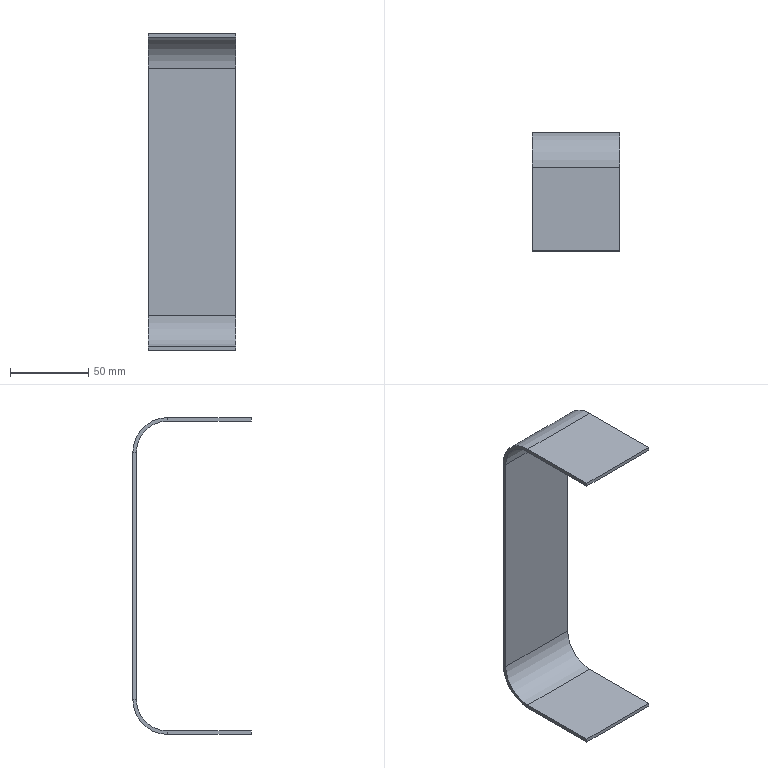Part | SolidWorks | features BaseBody 1, FlatPattern 1, SheetMetal 1, SolidToSheetMetal 1 | 1 solid | 22 faces | box 56 x 75.7 x 202.6 mm | volume 42664 mm3 | plane 18 | cylinder 4 | commonest cylinder face diameters 40 x2 44.6 x2
STEP:
#1=CARTESIAN_POINT('',(1097.7,32.3,248.9));
#2=VERTEX_POINT('',#1);
#3=CARTESIAN_POINT('',(1097.7,32.3,251.2));
#4=VERTEX_POINT('',#3);
#5=CARTESIAN_POINT('',(1097.7,32.3,251.2));
#6=DIRECTION('',(0.,0.,1.));
#7=VECTOR('',#6,1000.);
#8=LINE('',#5,#7);
#9=EDGE_CURVE('',#2,#4,#8,.T.);
#10=ORIENTED_EDGE('',*,*,#9,.F.);
#11=CARTESIAN_POINT('',(1153.7,32.3,248.9));
#12=VERTEX_POINT('',#11);
#13=CARTESIAN_POINT('',(1153.7,32.3,248.9));
#14=DIRECTION('',(-1.,0.,0.));
#15=VECTOR('',#14,1000.);
#16=LINE('',#13,#15);
#17=EDGE_CURVE('',#12,#2,#16,.T.);
#18=ORIENTED_EDGE('',*,*,#17,.F.);
#19=CARTESIAN_POINT('',(1153.7,32.3,251.2));
#20=VERTEX_POINT('',#19);
#21=CARTESIAN_POINT('',(1153.7,32.3,251.2));
#22=DIRECTION('',(0.,0.,1.));
#23=VECTOR('',#22,1000.);
#24=LINE('',#21,#23);
#25=EDGE_CURVE('',#12,#20,#24,.T.);
#26=ORIENTED_EDGE('',*,*,#25,.T.);
#27=CARTESIAN_POINT('',(1125.7,32.3,251.2));
#28=DIRECTION('',(-1.,0.,0.));
#29=VECTOR('',#28,1000.);
#30=LINE('',#27,#29);
#31=EDGE_CURVE('',#20,#4,#30,.T.);
#32=ORIENTED_EDGE('',*,*,#31,.T.);
#33=EDGE_LOOP('',(#10,#18,#26,#32));
#34=FACE_OUTER_BOUND('',#33,.T.);
#35=CARTESIAN_POINT('',(1125.7,32.3,251.2));
#36=DIRECTION('',(0.,-1.,0.));
#37=DIRECTION('',(-1.,0.,0.));
#38=AXIS2_PLACEMENT_3D('',#35,#36,#37);
#39=PLANE('',#38);
#40=ADVANCED_FACE('',(#34),#39,.T.);
#41=ORIENTED_EDGE('',*,*,#25,.F.);
#42=CARTESIAN_POINT('',(1153.7,85.7,248.9));
#43=VERTEX_POINT('',#42);
#44=CARTESIAN_POINT('',(1153.7,85.7,248.9));
#45=DIRECTION('',(0.,-1.,0.));
#46=VECTOR('',#45,1000.);
#47=LINE('',#44,#46);
#48=EDGE_CURVE('',#43,#12,#47,.T.);
#49=ORIENTED_EDGE('',*,*,#48,.F.);
#50=CARTESIAN_POINT('',(1153.7,85.7,251.2));
#51=VERTEX_POINT('',#50);
#52=CARTESIAN_POINT('',(1153.7,85.7,251.2));
#53=DIRECTION('',(0.,0.,1.));
#54=VECTOR('',#53,1000.);
#55=LINE('',#52,#54);
#56=EDGE_CURVE('',#43,#51,#55,.T.);
#57=ORIENTED_EDGE('',*,*,#56,.T.);
#58=CARTESIAN_POINT('',(1153.7,70.15,251.2));
#59=DIRECTION('',(0.,-1.,0.));
#60=VECTOR('',#59,1000.);
#61=LINE('',#58,#60);
#62=EDGE_CURVE('',#51,#20,#61,.T.);
#63=ORIENTED_EDGE('',*,*,#62,.T.);
#64=EDGE_LOOP('',(#41,#49,#57,#63));
#65=FACE_OUTER_BOUND('',#64,.T.);
#66=CARTESIAN_POINT('',(1153.7,70.15,251.2));
#67=DIRECTION('',(1.,0.,0.));
#68=DIRECTION('',(0.,-1.,0.));
#69=AXIS2_PLACEMENT_3D('',#66,#67,#68);
#70=PLANE('',#69);
#71=ADVANCED_FACE('',(#65),#70,.T.);
#72=ORIENTED_EDGE('',*,*,#56,.F.);
#73=CARTESIAN_POINT('',(1153.7,108.,271.2));
#74=VERTEX_POINT('',#73);
#75=CARTESIAN_POINT('',(1153.7,85.7,271.2));
#76=DIRECTION('',(-1.,0.,0.));
#77=DIRECTION('',(0.,0.,-1.));
#78=AXIS2_PLACEMENT_3D('',#75,#76,#77);
#79=CIRCLE('',#78,22.3);
#80=EDGE_CURVE('',#74,#43,#79,.T.);
#81=ORIENTED_EDGE('',*,*,#80,.F.);
#82=CARTESIAN_POINT('',(1153.7,105.7,271.2));
#83=VERTEX_POINT('',#82);
#84=CARTESIAN_POINT('',(1153.7,105.7,271.2));
#85=DIRECTION('',(0.,-1.,0.));
#86=VECTOR('',#85,1000.);
#87=LINE('',#84,#86);
#88=EDGE_CURVE('',#74,#83,#87,.T.);
#89=ORIENTED_EDGE('',*,*,#88,.T.);
#90=CARTESIAN_POINT('',(1153.7,85.7,271.2));
#91=DIRECTION('',(-1.,0.,0.));
#92=DIRECTION('',(0.,0.,-1.));
#93=AXIS2_PLACEMENT_3D('',#90,#91,#92);
#94=CIRCLE('',#93,20.);
#95=EDGE_CURVE('',#83,#51,#94,.T.);
#96=ORIENTED_EDGE('',*,*,#95,.T.);
#97=EDGE_LOOP('',(#72,#81,#89,#96));
#98=FACE_OUTER_BOUND('',#97,.T.);
#99=CARTESIAN_POINT('',(1153.7,85.7,271.2));
#100=DIRECTION('',(-1.,0.,0.));
#101=DIRECTION('',(0.,0.,1.));
#102=AXIS2_PLACEMENT_3D('',#99,#100,#101);
#103=PLANE('',#102);
#104=ADVANCED_FACE('',(#98),#103,.F.);
#105=ORIENTED_EDGE('',*,*,#88,.F.);
#106=CARTESIAN_POINT('',(1153.7,108.,429.2));
#107=VERTEX_POINT('',#106);
#108=CARTESIAN_POINT('',(1153.7,108.,429.2));
#109=DIRECTION('',(0.,0.,-1.));
#110=VECTOR('',#109,1000.);
#111=LINE('',#108,#110);
#112=EDGE_CURVE('',#107,#74,#111,.T.);
#113=ORIENTED_EDGE('',*,*,#112,.F.);
#114=CARTESIAN_POINT('',(1153.7,105.7,429.2));
#115=VERTEX_POINT('',#114);
#116=CARTESIAN_POINT('',(1153.7,105.7,429.2));
#117=DIRECTION('',(0.,-1.,0.));
#118=VECTOR('',#117,1000.);
#119=LINE('',#116,#118);
#120=EDGE_CURVE('',#107,#115,#119,.T.);
#121=ORIENTED_EDGE('',*,*,#120,.T.);
#122=CARTESIAN_POINT('',(1153.7,105.7,350.2));
#123=DIRECTION('',(0.,0.,-1.));
#124=VECTOR('',#123,1000.);
#125=LINE('',#122,#124);
#126=EDGE_CURVE('',#115,#83,#125,.T.);
#127=ORIENTED_EDGE('',*,*,#126,.T.);
#128=EDGE_LOOP('',(#105,#113,#121,#127));
#129=FACE_OUTER_BOUND('',#128,.T.);
#130=CARTESIAN_POINT('',(1153.7,105.7,350.2));
#131=DIRECTION('',(1.,0.,0.));
#132=DIRECTION('',(0.,0.,-1.));
#133=AXIS2_PLACEMENT_3D('',#130,#131,#132);
#134=PLANE('',#133);
#135=ADVANCED_FACE('',(#129),#134,.T.);
#136=ORIENTED_EDGE('',*,*,#120,.F.);
#137=CARTESIAN_POINT('',(1153.7,85.7,451.5));
#138=VERTEX_POINT('',#137);
#139=CARTESIAN_POINT('',(1153.7,85.7,429.2));
#140=DIRECTION('',(1.,0.,0.));
#141=DIRECTION('',(0.,0.,-1.));
#142=AXIS2_PLACEMENT_3D('',#139,#140,#141);
#143=CIRCLE('',#142,22.3);
#144=EDGE_CURVE('',#107,#138,#143,.T.);
#145=ORIENTED_EDGE('',*,*,#144,.T.);
#146=CARTESIAN_POINT('',(1153.7,85.7,449.2));
#147=VERTEX_POINT('',#146);
#148=CARTESIAN_POINT('',(1153.7,85.7,449.2));
#149=DIRECTION('',(0.,0.,-1.));
#150=VECTOR('',#149,1000.);
#151=LINE('',#148,#150);
#152=EDGE_CURVE('',#138,#147,#151,.T.);
#153=ORIENTED_EDGE('',*,*,#152,.T.);
#154=CARTESIAN_POINT('',(1153.7,85.7,429.2));
#155=DIRECTION('',(1.,0.,0.));
#156=DIRECTION('',(0.,0.,-1.));
#157=AXIS2_PLACEMENT_3D('',#154,#155,#156);
#158=CIRCLE('',#157,20.);
#159=EDGE_CURVE('',#115,#147,#158,.T.);
#160=ORIENTED_EDGE('',*,*,#159,.F.);
#161=EDGE_LOOP('',(#136,#145,#153,#160));
#162=FACE_OUTER_BOUND('',#161,.T.);
#163=CARTESIAN_POINT('',(1153.7,85.7,429.2));
#164=DIRECTION('',(-1.,0.,0.));
#165=DIRECTION('',(0.,0.,1.));
#166=AXIS2_PLACEMENT_3D('',#163,#164,#165);
#167=PLANE('',#166);
#168=ADVANCED_FACE('',(#162),#167,.F.);
#169=ORIENTED_EDGE('',*,*,#152,.F.);
#170=CARTESIAN_POINT('',(1153.7,32.3,451.5));
#171=VERTEX_POINT('',#170);
#172=CARTESIAN_POINT('',(1153.7,32.3,451.5));
#173=DIRECTION('',(0.,1.,0.));
#174=VECTOR('',#173,1000.);
#175=LINE('',#172,#174);
#176=EDGE_CURVE('',#171,#138,#175,.T.);
#177=ORIENTED_EDGE('',*,*,#176,.F.);
#178=CARTESIAN_POINT('',(1153.7,32.3,449.2));
#179=VERTEX_POINT('',#178);
#180=CARTESIAN_POINT('',(1153.7,32.3,449.2));
#181=DIRECTION('',(0.,0.,-1.));
#182=VECTOR('',#181,1000.);
#183=LINE('',#180,#182);
#184=EDGE_CURVE('',#171,#179,#183,.T.);
#185=ORIENTED_EDGE('',*,*,#184,.T.);
#186=CARTESIAN_POINT('',(1153.7,59.,449.2));
#187=DIRECTION('',(0.,1.,0.));
#188=VECTOR('',#187,1000.);
#189=LINE('',#186,#188);
#190=EDGE_CURVE('',#179,#147,#189,.T.);
#191=ORIENTED_EDGE('',*,*,#190,.T.);
#192=EDGE_LOOP('',(#169,#177,#185,#191));
#193=FACE_OUTER_BOUND('',#192,.T.);
#194=CARTESIAN_POINT('',(1153.7,59.,449.2));
#195=DIRECTION('',(1.,0.,0.));
#196=DIRECTION('',(0.,1.,0.));
#197=AXIS2_PLACEMENT_3D('',#194,#195,#196);
#198=PLANE('',#197);
#199=ADVANCED_FACE('',(#193),#198,.T.);
#200=ORIENTED_EDGE('',*,*,#184,.F.);
#201=CARTESIAN_POINT('',(1097.7,32.3,451.5));
#202=VERTEX_POINT('',#201);
#203=CARTESIAN_POINT('',(1097.7,32.3,451.5));
#204=DIRECTION('',(1.,0.,0.));
#205=VECTOR('',#204,1000.);
#206=LINE('',#203,#205);
#207=EDGE_CURVE('',#202,#171,#206,.T.);
#208=ORIENTED_EDGE('',*,*,#207,.F.);
#209=CARTESIAN_POINT('',(1097.7,32.3,449.2));
#210=VERTEX_POINT('',#209);
#211=CARTESIAN_POINT('',(1097.7,32.3,449.2));
#212=DIRECTION('',(0.,0.,-1.));
#213=VECTOR('',#212,1000.);
#214=LINE('',#211,#213);
#215=EDGE_CURVE('',#202,#210,#214,.T.);
#216=ORIENTED_EDGE('',*,*,#215,.T.);
#217=CARTESIAN_POINT('',(1125.7,32.3,449.2));
#218=DIRECTION('',(1.,0.,0.));
#219=VECTOR('',#218,1000.);
#220=LINE('',#217,#219);
#221=EDGE_CURVE('',#210,#179,#220,.T.);
#222=ORIENTED_EDGE('',*,*,#221,.T.);
#223=EDGE_LOOP('',(#200,#208,#216,#222));
#224=FACE_OUTER_BOUND('',#223,.T.);
#225=CARTESIAN_POINT('',(1125.7,32.3,449.2));
#226=DIRECTION('',(0.,-1.,0.));
#227=DIRECTION('',(1.,0.,0.));
#228=AXIS2_PLACEMENT_3D('',#225,#226,#227);
#229=PLANE('',#228);
#230=ADVANCED_FACE('',(#224),#229,.T.);
#231=ORIENTED_EDGE('',*,*,#215,.F.);
#232=CARTESIAN_POINT('',(1097.7,85.7,451.5));
#233=VERTEX_POINT('',#232);
#234=CARTESIAN_POINT('',(1097.7,32.3,451.5));
#235=DIRECTION('',(0.,-1.,0.));
#236=VECTOR('',#235,1000.);
#237=LINE('',#234,#236);
#238=EDGE_CURVE('',#233,#202,#237,.T.);
#239=ORIENTED_EDGE('',*,*,#238,.F.);
#240=CARTESIAN_POINT('',(1097.7,85.7,449.2));
#241=VERTEX_POINT('',#240);
#242=CARTESIAN_POINT('',(1097.7,85.7,449.2));
#243=DIRECTION('',(0.,0.,-1.));
#244=VECTOR('',#243,1000.);
#245=LINE('',#242,#244);
#246=EDGE_CURVE('',#233,#241,#245,.T.);
#247=ORIENTED_EDGE('',*,*,#246,.T.);
#248=CARTESIAN_POINT('',(1097.7,59.,449.2));
#249=DIRECTION('',(0.,-1.,0.));
#250=VECTOR('',#249,1000.);
#251=LINE('',#248,#250);
#252=EDGE_CURVE('',#241,#210,#251,.T.);
#253=ORIENTED_EDGE('',*,*,#252,.T.);
#254=EDGE_LOOP('',(#231,#239,#247,#253));
#255=FACE_OUTER_BOUND('',#254,.T.);
#256=CARTESIAN_POINT('',(1097.7,59.,449.2));
#257=DIRECTION('',(-1.,0.,0.));
#258=DIRECTION('',(0.,-1.,0.));
#259=AXIS2_PLACEMENT_3D('',#256,#257,#258);
#260=PLANE('',#259);
#261=ADVANCED_FACE('',(#255),#260,.T.);
#262=ORIENTED_EDGE('',*,*,#246,.F.);
#263=CARTESIAN_POINT('',(1097.7,108.,429.2));
#264=VERTEX_POINT('',#263);
#265=CARTESIAN_POINT('',(1097.7,85.7,429.2));
#266=DIRECTION('',(-1.,0.,0.));
#267=DIRECTION('',(0.,0.,-1.));
#268=AXIS2_PLACEMENT_3D('',#265,#266,#267);
#269=CIRCLE('',#268,22.3);
#270=EDGE_CURVE('',#233,#264,#269,.T.);
#271=ORIENTED_EDGE('',*,*,#270,.T.);
#272=CARTESIAN_POINT('',(1097.7,105.7,429.2));
#273=VERTEX_POINT('',#272);
#274=CARTESIAN_POINT('',(1097.7,105.7,429.2));
#275=DIRECTION('',(0.,-1.,0.));
#276=VECTOR('',#275,1000.);
#277=LINE('',#274,#276);
#278=EDGE_CURVE('',#264,#273,#277,.T.);
#279=ORIENTED_EDGE('',*,*,#278,.T.);
#280=CARTESIAN_POINT('',(1097.7,85.7,429.2));
#281=DIRECTION('',(-1.,0.,0.));
#282=DIRECTION('',(0.,0.,-1.));
#283=AXIS2_PLACEMENT_3D('',#280,#281,#282);
#284=CIRCLE('',#283,20.);
#285=EDGE_CURVE('',#241,#273,#284,.T.);
#286=ORIENTED_EDGE('',*,*,#285,.F.);
#287=EDGE_LOOP('',(#262,#271,#279,#286));
#288=FACE_OUTER_BOUND('',#287,.T.);
#289=CARTESIAN_POINT('',(1097.7,85.7,429.2));
#290=DIRECTION('',(-1.,0.,0.));
#291=DIRECTION('',(0.,0.,1.));
#292=AXIS2_PLACEMENT_3D('',#289,#290,#291);
#293=PLANE('',#292);
#294=ADVANCED_FACE('',(#288),#293,.T.);
#295=ORIENTED_EDGE('',*,*,#278,.F.);
#296=CARTESIAN_POINT('',(1097.7,108.,271.2));
#297=VERTEX_POINT('',#296);
#298=CARTESIAN_POINT('',(1097.7,108.,429.2));
#299=DIRECTION('',(0.,0.,-1.));
#300=VECTOR('',#299,1000.);
#301=LINE('',#298,#300);
#302=EDGE_CURVE('',#264,#297,#301,.T.);
#303=ORIENTED_EDGE('',*,*,#302,.T.);
#304=CARTESIAN_POINT('',(1097.7,105.7,271.2));
#305=VERTEX_POINT('',#304);
#306=CARTESIAN_POINT('',(1097.7,105.7,271.2));
#307=DIRECTION('',(0.,-1.,0.));
#308=VECTOR('',#307,1000.);
#309=LINE('',#306,#308);
#310=EDGE_CURVE('',#297,#305,#309,.T.);
#311=ORIENTED_EDGE('',*,*,#310,.T.);
#312=CARTESIAN_POINT('',(1097.7,105.7,350.2));
#313=DIRECTION('',(0.,0.,-1.));
#314=VECTOR('',#313,1000.);
#315=LINE('',#312,#314);
#316=EDGE_CURVE('',#273,#305,#315,.T.);
#317=ORIENTED_EDGE('',*,*,#316,.F.);
#318=EDGE_LOOP('',(#295,#303,#311,#317));
#319=FACE_OUTER_BOUND('',#318,.T.);
#320=CARTESIAN_POINT('',(1097.7,105.7,350.2));
#321=DIRECTION('',(1.,0.,0.));
#322=DIRECTION('',(0.,0.,-1.));
#323=AXIS2_PLACEMENT_3D('',#320,#321,#322);
#324=PLANE('',#323);
#325=ADVANCED_FACE('',(#319),#324,.F.);
#326=ORIENTED_EDGE('',*,*,#310,.F.);
#327=CARTESIAN_POINT('',(1097.7,85.7,248.9));
#328=VERTEX_POINT('',#327);
#329=CARTESIAN_POINT('',(1097.7,85.7,271.2));
#330=DIRECTION('',(-1.,0.,0.));
#331=DIRECTION('',(0.,0.,-1.));
#332=AXIS2_PLACEMENT_3D('',#329,#330,#331);
#333=CIRCLE('',#332,22.3);
#334=EDGE_CURVE('',#297,#328,#333,.T.);
#335=ORIENTED_EDGE('',*,*,#334,.T.);
#336=CARTESIAN_POINT('',(1097.7,85.7,251.2));
#337=VERTEX_POINT('',#336);
#338=CARTESIAN_POINT('',(1097.7,85.7,251.2));
#339=DIRECTION('',(0.,0.,1.));
#340=VECTOR('',#339,1000.);
#341=LINE('',#338,#340);
#342=EDGE_CURVE('',#328,#337,#341,.T.);
#343=ORIENTED_EDGE('',*,*,#342,.T.);
#344=CARTESIAN_POINT('',(1097.7,85.7,271.2));
#345=DIRECTION('',(-1.,0.,0.));
#346=DIRECTION('',(0.,0.,-1.));
#347=AXIS2_PLACEMENT_3D('',#344,#345,#346);
#348=CIRCLE('',#347,20.);
#349=EDGE_CURVE('',#305,#337,#348,.T.);
#350=ORIENTED_EDGE('',*,*,#349,.F.);
#351=EDGE_LOOP('',(#326,#335,#343,#350));
#352=FACE_OUTER_BOUND('',#351,.T.);
#353=CARTESIAN_POINT('',(1097.7,85.7,271.2));
#354=DIRECTION('',(-1.,0.,0.));
#355=DIRECTION('',(0.,0.,1.));
#356=AXIS2_PLACEMENT_3D('',#353,#354,#355);
#357=PLANE('',#356);
#358=ADVANCED_FACE('',(#352),#357,.T.);
#359=CARTESIAN_POINT('',(1097.7,85.7,248.9));
#360=DIRECTION('',(0.,-1.,0.));
#361=VECTOR('',#360,1000.);
#362=LINE('',#359,#361);
#363=EDGE_CURVE('',#328,#2,#362,.T.);
#364=ORIENTED_EDGE('',*,*,#363,.T.);
#365=ORIENTED_EDGE('',*,*,#9,.T.);
#366=CARTESIAN_POINT('',(1097.7,70.15,251.2));
#367=DIRECTION('',(0.,-1.,0.));
#368=VECTOR('',#367,1000.);
#369=LINE('',#366,#368);
#370=EDGE_CURVE('',#337,#4,#369,.T.);
#371=ORIENTED_EDGE('',*,*,#370,.F.);
#372=ORIENTED_EDGE('',*,*,#342,.F.);
#373=EDGE_LOOP('',(#364,#365,#371,#372));
#374=FACE_OUTER_BOUND('',#373,.T.);
#375=CARTESIAN_POINT('',(1097.7,70.15,251.2));
#376=DIRECTION('',(1.,0.,0.));
#377=DIRECTION('',(0.,-1.,0.));
#378=AXIS2_PLACEMENT_3D('',#375,#376,#377);
#379=PLANE('',#378);
#380=ADVANCED_FACE('',(#374),#379,.F.);
#381=CARTESIAN_POINT('',(1125.7,105.7,271.2));
#382=DIRECTION('',(-1.,0.,0.));
#383=VECTOR('',#382,1000.);
#384=LINE('',#381,#383);
#385=EDGE_CURVE('',#83,#305,#384,.T.);
#386=ORIENTED_EDGE('',*,*,#385,.T.);
#387=ORIENTED_EDGE('',*,*,#349,.T.);
#388=CARTESIAN_POINT('',(1125.7,85.7,251.2));
#389=DIRECTION('',(1.,0.,0.));
#390=VECTOR('',#389,1000.);
#391=LINE('',#388,#390);
#392=EDGE_CURVE('',#337,#51,#391,.T.);
#393=ORIENTED_EDGE('',*,*,#392,.T.);
#394=ORIENTED_EDGE('',*,*,#95,.F.);
#395=EDGE_LOOP('',(#386,#387,#393,#394));
#396=FACE_OUTER_BOUND('',#395,.T.);
#397=CARTESIAN_POINT('',(1097.7,85.7,271.2));
#398=DIRECTION('',(1.,0.,0.));
#399=DIRECTION('',(0.,0.,-1.));
#400=AXIS2_PLACEMENT_3D('',#397,#398,#399);
#401=CYLINDRICAL_SURFACE('',#400,20.);
#402=ADVANCED_FACE('',(#396),#401,.F.);
#403=ORIENTED_EDGE('',*,*,#62,.F.);
#404=ORIENTED_EDGE('',*,*,#392,.F.);
#405=ORIENTED_EDGE('',*,*,#370,.T.);
#406=ORIENTED_EDGE('',*,*,#31,.F.);
#407=EDGE_LOOP('',(#403,#404,#405,#406));
#408=FACE_OUTER_BOUND('',#407,.T.);
#409=CARTESIAN_POINT('',(1153.7,85.7,251.2));
#410=DIRECTION('',(0.,0.,-1.));
#411=DIRECTION('',(0.,-1.,0.));
#412=AXIS2_PLACEMENT_3D('',#409,#410,#411);
#413=PLANE('',#412);
#414=ADVANCED_FACE('',(#408),#413,.F.);
#415=CARTESIAN_POINT('',(1125.7,85.7,449.2));
#416=DIRECTION('',(-1.,0.,0.));
#417=VECTOR('',#416,1000.);
#418=LINE('',#415,#417);
#419=EDGE_CURVE('',#147,#241,#418,.T.);
#420=ORIENTED_EDGE('',*,*,#419,.T.);
#421=ORIENTED_EDGE('',*,*,#285,.T.);
#422=CARTESIAN_POINT('',(1125.7,105.7,429.2));
#423=DIRECTION('',(1.,0.,0.));
#424=VECTOR('',#423,1000.);
#425=LINE('',#422,#424);
#426=EDGE_CURVE('',#273,#115,#425,.T.);
#427=ORIENTED_EDGE('',*,*,#426,.T.);
#428=ORIENTED_EDGE('',*,*,#159,.T.);
#429=EDGE_LOOP('',(#420,#421,#427,#428));
#430=FACE_OUTER_BOUND('',#429,.T.);
#431=CARTESIAN_POINT('',(1097.7,85.7,429.2));
#432=DIRECTION('',(1.,0.,0.));
#433=DIRECTION('',(0.,0.,-1.));
#434=AXIS2_PLACEMENT_3D('',#431,#432,#433);
#435=CYLINDRICAL_SURFACE('',#434,20.);
#436=ADVANCED_FACE('',(#430),#435,.F.);
#437=ORIENTED_EDGE('',*,*,#126,.F.);
#438=ORIENTED_EDGE('',*,*,#426,.F.);
#439=ORIENTED_EDGE('',*,*,#316,.T.);
#440=ORIENTED_EDGE('',*,*,#385,.F.);
#441=EDGE_LOOP('',(#437,#438,#439,#440));
#442=FACE_OUTER_BOUND('',#441,.T.);
#443=CARTESIAN_POINT('',(1097.7,105.7,429.2));
#444=DIRECTION('',(0.,1.,0.));
#445=DIRECTION('',(1.,0.,0.));
#446=AXIS2_PLACEMENT_3D('',#443,#444,#445);
#447=PLANE('',#446);
#448=ADVANCED_FACE('',(#442),#447,.F.);
#449=ORIENTED_EDGE('',*,*,#190,.F.);
#450=ORIENTED_EDGE('',*,*,#221,.F.);
#451=ORIENTED_EDGE('',*,*,#252,.F.);
#452=ORIENTED_EDGE('',*,*,#419,.F.);
#453=EDGE_LOOP('',(#449,#450,#451,#452));
#454=FACE_OUTER_BOUND('',#453,.T.);
#455=CARTESIAN_POINT('',(1097.7,32.3,449.2));
#456=DIRECTION('',(0.,0.,1.));
#457=DIRECTION('',(1.,0.,0.));
#458=AXIS2_PLACEMENT_3D('',#455,#456,#457);
#459=PLANE('',#458);
#460=ADVANCED_FACE('',(#454),#459,.F.);
#461=CARTESIAN_POINT('',(1097.7,108.,271.2));
#462=DIRECTION('',(-1.,0.,0.));
#463=VECTOR('',#462,1000.);
#464=LINE('',#461,#463);
#465=EDGE_CURVE('',#74,#297,#464,.T.);
#466=ORIENTED_EDGE('',*,*,#465,.F.);
#467=ORIENTED_EDGE('',*,*,#80,.T.);
#468=CARTESIAN_POINT('',(1097.7,85.7,248.9));
#469=DIRECTION('',(1.,0.,0.));
#470=VECTOR('',#469,1000.);
#471=LINE('',#468,#470);
#472=EDGE_CURVE('',#328,#43,#471,.T.);
#473=ORIENTED_EDGE('',*,*,#472,.F.);
#474=ORIENTED_EDGE('',*,*,#334,.F.);
#475=EDGE_LOOP('',(#466,#467,#473,#474));
#476=FACE_OUTER_BOUND('',#475,.T.);
#477=CARTESIAN_POINT('',(1097.7,85.7,271.2));
#478=DIRECTION('',(1.,0.,0.));
#479=DIRECTION('',(0.,0.,-1.));
#480=AXIS2_PLACEMENT_3D('',#477,#478,#479);
#481=CYLINDRICAL_SURFACE('',#480,22.3);
#482=ADVANCED_FACE('',(#476),#481,.T.);
#483=ORIENTED_EDGE('',*,*,#48,.T.);
#484=ORIENTED_EDGE('',*,*,#17,.T.);
#485=ORIENTED_EDGE('',*,*,#363,.F.);
#486=ORIENTED_EDGE('',*,*,#472,.T.);
#487=EDGE_LOOP('',(#483,#484,#485,#486));
#488=FACE_OUTER_BOUND('',#487,.T.);
#489=CARTESIAN_POINT('',(1153.7,85.7,248.9));
#490=DIRECTION('',(0.,0.,-1.));
#491=DIRECTION('',(0.,-1.,0.));
#492=AXIS2_PLACEMENT_3D('',#489,#490,#491);
#493=PLANE('',#492);
#494=ADVANCED_FACE('',(#488),#493,.T.);
#495=CARTESIAN_POINT('',(1097.7,85.7,451.5));
#496=DIRECTION('',(-1.,0.,0.));
#497=VECTOR('',#496,1000.);
#498=LINE('',#495,#497);
#499=EDGE_CURVE('',#138,#233,#498,.T.);
#500=ORIENTED_EDGE('',*,*,#499,.F.);
#501=ORIENTED_EDGE('',*,*,#144,.F.);
#502=CARTESIAN_POINT('',(1097.7,108.,429.2));
#503=DIRECTION('',(1.,0.,0.));
#504=VECTOR('',#503,1000.);
#505=LINE('',#502,#504);
#506=EDGE_CURVE('',#264,#107,#505,.T.);
#507=ORIENTED_EDGE('',*,*,#506,.F.);
#508=ORIENTED_EDGE('',*,*,#270,.F.);
#509=EDGE_LOOP('',(#500,#501,#507,#508));
#510=FACE_OUTER_BOUND('',#509,.T.);
#511=CARTESIAN_POINT('',(1097.7,85.7,429.2));
#512=DIRECTION('',(1.,0.,0.));
#513=DIRECTION('',(0.,0.,-1.));
#514=AXIS2_PLACEMENT_3D('',#511,#512,#513);
#515=CYLINDRICAL_SURFACE('',#514,22.3);
#516=ADVANCED_FACE('',(#510),#515,.T.);
#517=ORIENTED_EDGE('',*,*,#112,.T.);
#518=ORIENTED_EDGE('',*,*,#465,.T.);
#519=ORIENTED_EDGE('',*,*,#302,.F.);
#520=ORIENTED_EDGE('',*,*,#506,.T.);
#521=EDGE_LOOP('',(#517,#518,#519,#520));
#522=FACE_OUTER_BOUND('',#521,.T.);
#523=CARTESIAN_POINT('',(1097.7,108.,429.2));
#524=DIRECTION('',(0.,1.,0.));
#525=DIRECTION('',(1.,0.,0.));
#526=AXIS2_PLACEMENT_3D('',#523,#524,#525);
#527=PLANE('',#526);
#528=ADVANCED_FACE('',(#522),#527,.T.);
#529=ORIENTED_EDGE('',*,*,#176,.T.);
#530=ORIENTED_EDGE('',*,*,#499,.T.);
#531=ORIENTED_EDGE('',*,*,#238,.T.);
#532=ORIENTED_EDGE('',*,*,#207,.T.);
#533=EDGE_LOOP('',(#529,#530,#531,#532));
#534=FACE_OUTER_BOUND('',#533,.T.);
#535=CARTESIAN_POINT('',(1097.7,32.3,451.5));
#536=DIRECTION('',(0.,0.,1.));
#537=DIRECTION('',(1.,0.,0.));
#538=AXIS2_PLACEMENT_3D('',#535,#536,#537);
#539=PLANE('',#538);
#540=ADVANCED_FACE('',(#534),#539,.T.);
#541=CLOSED_SHELL('',(#40,#71,#104,#135,#168,#199,#230,#261,#294,#325,#358,#380,#402,#414,#436,#448,#460,#482,#494,#516,#528,#540));
#542=MANIFOLD_SOLID_BREP('',#541);
#543=CARTESIAN_POINT('',(0.,0.,0.));
#544=DIRECTION('',(0.,0.,1.));
#545=DIRECTION('',(1.,0.,0.));
#546=AXIS2_PLACEMENT_3D('',#543,#544,#545);
#547=(LENGTH_UNIT()NAMED_UNIT(*)SI_UNIT(.MILLI.,.METRE.));
#548=UNCERTAINTY_MEASURE_WITH_UNIT(LENGTH_MEASURE(0.00001),#547,'','');
#549=(NAMED_UNIT(*)PLANE_ANGLE_UNIT()SI_UNIT($,.RADIAN.));
#550=(NAMED_UNIT(*)SI_UNIT($,.STERADIAN.)SOLID_ANGLE_UNIT());
#551=(GEOMETRIC_REPRESENTATION_CONTEXT(3)GLOBAL_UNCERTAINTY_ASSIGNED_CONTEXT((#548))GLOBAL_UNIT_ASSIGNED_CONTEXT((#547,#549,#550))REPRESENTATION_CONTEXT('',''));
#552=ADVANCED_BREP_SHAPE_REPRESENTATION('',(#542,#546),#551);